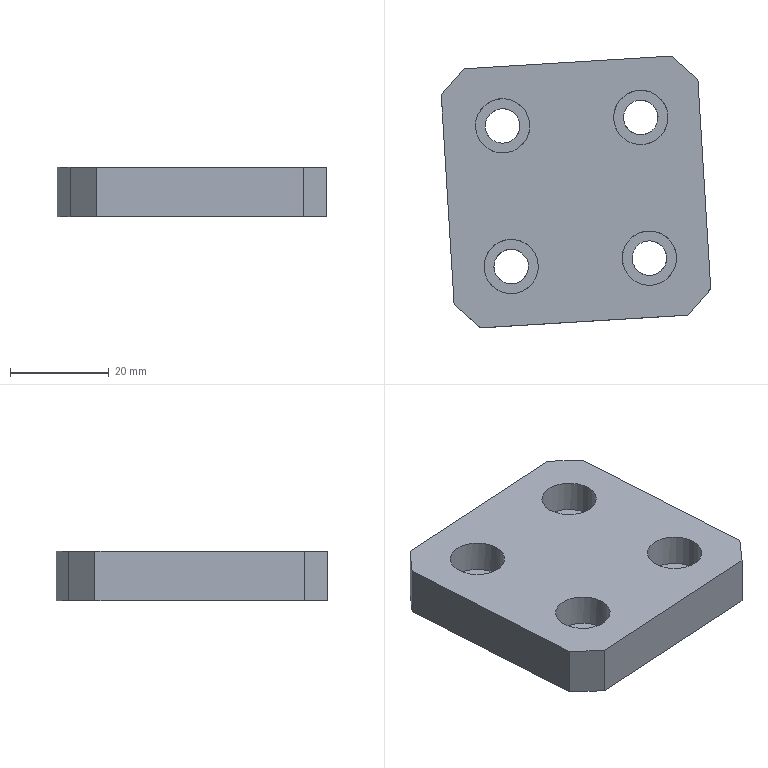Part | STEP file | 车灯-后视镜_id138_x_t | 1 solid | 22 faces | box 54.498 x 54.966 x 10 mm | volume 23790 mm3 | plane 14 | cylinder 8 | commonest cylinder face diameters 7 x4 11 x4
STEP:
#1=CARTESIAN_POINT('',(118.099,33.063,-255.5));
#2=VERTEX_POINT('',#1);
#3=CARTESIAN_POINT('',(120.693,-9.358,-255.5));
#4=VERTEX_POINT('',#3);
#5=CARTESIAN_POINT('',(119.355,12.524,-255.5));
#6=DIRECTION('',(0.06105,-0.9981,0.));
#7=VECTOR('',#6,1.);
#8=LINE('',#5,#7);
#9=EDGE_CURVE('',#2,#4,#8,.T.);
#10=ORIENTED_EDGE('',*,*,#9,.F.);
#11=CARTESIAN_POINT('',(112.803,37.748,-255.5));
#12=VERTEX_POINT('',#11);
#13=CARTESIAN_POINT('',(107.277,42.637,-255.5));
#14=DIRECTION('',(-0.749,0.6626,0.));
#15=VECTOR('',#14,1.);
#16=LINE('',#13,#15);
#17=EDGE_CURVE('',#2,#12,#16,.T.);
#18=ORIENTED_EDGE('',*,*,#17,.T.);
#19=CARTESIAN_POINT('',(70.881,35.184,-255.5));
#20=VERTEX_POINT('',#19);
#21=CARTESIAN_POINT('',(76.858,35.55,-255.5));
#22=DIRECTION('',(0.9981,0.06105,0.));
#23=VECTOR('',#22,1.);
#24=LINE('',#21,#23);
#25=EDGE_CURVE('',#20,#12,#24,.T.);
#26=ORIENTED_EDGE('',*,*,#25,.F.);
#27=CARTESIAN_POINT('',(66.196,29.888,-255.5));
#28=VERTEX_POINT('',#27);
#29=CARTESIAN_POINT('',(61.703,24.81,-255.5));
#30=DIRECTION('',(-0.6626,-0.749,0.));
#31=VECTOR('',#30,1.);
#32=LINE('',#29,#31);
#33=EDGE_CURVE('',#20,#28,#32,.T.);
#34=ORIENTED_EDGE('',*,*,#33,.T.);
#35=CARTESIAN_POINT('',(68.79,-12.533,-255.5));
#36=VERTEX_POINT('',#35);
#37=CARTESIAN_POINT('',(67.452,9.349,-255.5));
#38=DIRECTION('',(-0.06105,0.9981,0.));
#39=VECTOR('',#38,1.);
#40=LINE('',#37,#39);
#41=EDGE_CURVE('',#36,#28,#40,.T.);
#42=ORIENTED_EDGE('',*,*,#41,.F.);
#43=CARTESIAN_POINT('',(74.086,-17.218,-255.5));
#44=VERTEX_POINT('',#43);
#45=CARTESIAN_POINT('',(63.,-7.409,-255.5));
#46=DIRECTION('',(0.749,-0.6626,0.));
#47=VECTOR('',#46,1.);
#48=LINE('',#45,#47);
#49=EDGE_CURVE('',#36,#44,#48,.T.);
#50=ORIENTED_EDGE('',*,*,#49,.T.);
#51=CARTESIAN_POINT('',(116.008,-14.654,-255.5));
#52=VERTEX_POINT('',#51);
#53=CARTESIAN_POINT('',(80.063,-16.853,-255.5));
#54=DIRECTION('',(-0.9981,-0.06105,0.));
#55=VECTOR('',#54,1.);
#56=LINE('',#53,#55);
#57=EDGE_CURVE('',#52,#44,#56,.T.);
#58=ORIENTED_EDGE('',*,*,#57,.F.);
#59=CARTESIAN_POINT('',(111.749,-19.467,-255.5));
#60=DIRECTION('',(0.6626,0.749,0.));
#61=VECTOR('',#60,1.);
#62=LINE('',#59,#61);
#63=EDGE_CURVE('',#52,#4,#62,.T.);
#64=ORIENTED_EDGE('',*,*,#63,.T.);
#65=EDGE_LOOP('',(#10,#18,#26,#34,#42,#50,#58,#64));
#66=FACE_BOUND('',#65,.T.);
#67=CARTESIAN_POINT('',(85.841,-4.813,-255.5));
#68=VERTEX_POINT('',#67);
#69=CARTESIAN_POINT('',(80.341,-4.813,-255.5));
#70=DIRECTION('',(0.,0.,1.));
#71=DIRECTION('',(1.,0.,0.));
#72=AXIS2_PLACEMENT_3D('',#69,#70,#71);
#73=CIRCLE('',#72,5.5);
#74=EDGE_CURVE('',#68,#68,#73,.T.);
#75=ORIENTED_EDGE('',*,*,#74,.F.);
#76=EDGE_LOOP('',(#75));
#77=FACE_BOUND('',#76,.T.);
#78=CARTESIAN_POINT('',(113.788,-3.104,-255.5));
#79=VERTEX_POINT('',#78);
#80=CARTESIAN_POINT('',(108.288,-3.104,-255.5));
#81=DIRECTION('',(0.,0.,-1.));
#82=DIRECTION('',(1.,0.,0.));
#83=AXIS2_PLACEMENT_3D('',#80,#81,#82);
#84=CIRCLE('',#83,5.5);
#85=EDGE_CURVE('',#79,#79,#84,.T.);
#86=ORIENTED_EDGE('',*,*,#85,.T.);
#87=EDGE_LOOP('',(#86));
#88=FACE_BOUND('',#87,.T.);
#89=CARTESIAN_POINT('',(84.101,23.634,-255.5));
#90=VERTEX_POINT('',#89);
#91=CARTESIAN_POINT('',(78.601,23.634,-255.5));
#92=DIRECTION('',(0.,0.,-1.));
#93=DIRECTION('',(1.,0.,0.));
#94=AXIS2_PLACEMENT_3D('',#91,#92,#93);
#95=CIRCLE('',#94,5.5);
#96=EDGE_CURVE('',#90,#90,#95,.T.);
#97=ORIENTED_EDGE('',*,*,#96,.T.);
#98=EDGE_LOOP('',(#97));
#99=FACE_BOUND('',#98,.T.);
#100=CARTESIAN_POINT('',(112.049,25.343,-255.5));
#101=VERTEX_POINT('',#100);
#102=CARTESIAN_POINT('',(106.549,25.343,-255.5));
#103=DIRECTION('',(0.,0.,1.));
#104=DIRECTION('',(1.,0.,0.));
#105=AXIS2_PLACEMENT_3D('',#102,#103,#104);
#106=CIRCLE('',#105,5.5);
#107=EDGE_CURVE('',#101,#101,#106,.T.);
#108=ORIENTED_EDGE('',*,*,#107,.F.);
#109=EDGE_LOOP('',(#108));
#110=FACE_BOUND('',#109,.T.);
#111=CARTESIAN_POINT('',(78.42,10.02,-255.5));
#112=DIRECTION('',(0.,0.,1.));
#113=DIRECTION('',(0.9981,0.06105,0.));
#114=AXIS2_PLACEMENT_3D('',#111,#112,#113);
#115=PLANE('',#114);
#116=ADVANCED_FACE('',(#66,#77,#88,#99,#110),#115,.T.);
#117=CARTESIAN_POINT('',(74.086,-17.218,-265.5));
#118=VERTEX_POINT('',#117);
#119=CARTESIAN_POINT('',(116.008,-14.654,-265.5));
#120=VERTEX_POINT('',#119);
#121=CARTESIAN_POINT('',(80.063,-16.853,-265.5));
#122=DIRECTION('',(0.9981,0.06105,0.));
#123=VECTOR('',#122,1.);
#124=LINE('',#121,#123);
#125=EDGE_CURVE('',#118,#120,#124,.T.);
#126=ORIENTED_EDGE('',*,*,#125,.T.);
#127=CARTESIAN_POINT('',(116.008,-14.654,-267.5));
#128=DIRECTION('',(0.,0.,1.));
#129=VECTOR('',#128,1.);
#130=LINE('',#127,#129);
#131=EDGE_CURVE('',#120,#52,#130,.T.);
#132=ORIENTED_EDGE('',*,*,#131,.T.);
#133=ORIENTED_EDGE('',*,*,#57,.T.);
#134=CARTESIAN_POINT('',(74.086,-17.218,-267.5));
#135=DIRECTION('',(0.,0.,-1.));
#136=VECTOR('',#135,1.);
#137=LINE('',#134,#136);
#138=EDGE_CURVE('',#44,#118,#137,.T.);
#139=ORIENTED_EDGE('',*,*,#138,.T.);
#140=EDGE_LOOP('',(#126,#132,#133,#139));
#141=FACE_OUTER_BOUND('',#140,.T.);
#142=CARTESIAN_POINT('',(80.063,-16.853,-267.5));
#143=DIRECTION('',(0.06105,-0.9981,0.));
#144=DIRECTION('',(0.,0.,-1.));
#145=AXIS2_PLACEMENT_3D('',#142,#143,#144);
#146=PLANE('',#145);
#147=ADVANCED_FACE('',(#141),#146,.T.);
#148=ORIENTED_EDGE('',*,*,#25,.T.);
#149=CARTESIAN_POINT('',(112.803,37.748,-265.5));
#150=VERTEX_POINT('',#149);
#151=CARTESIAN_POINT('',(112.803,37.748,-267.5));
#152=DIRECTION('',(0.,0.,-1.));
#153=VECTOR('',#152,1.);
#154=LINE('',#151,#153);
#155=EDGE_CURVE('',#12,#150,#154,.T.);
#156=ORIENTED_EDGE('',*,*,#155,.T.);
#157=CARTESIAN_POINT('',(70.881,35.184,-265.5));
#158=VERTEX_POINT('',#157);
#159=CARTESIAN_POINT('',(76.858,35.55,-265.5));
#160=DIRECTION('',(-0.9981,-0.06105,0.));
#161=VECTOR('',#160,1.);
#162=LINE('',#159,#161);
#163=EDGE_CURVE('',#150,#158,#162,.T.);
#164=ORIENTED_EDGE('',*,*,#163,.T.);
#165=CARTESIAN_POINT('',(70.881,35.184,-267.5));
#166=DIRECTION('',(0.,0.,1.));
#167=VECTOR('',#166,1.);
#168=LINE('',#165,#167);
#169=EDGE_CURVE('',#158,#20,#168,.T.);
#170=ORIENTED_EDGE('',*,*,#169,.T.);
#171=EDGE_LOOP('',(#148,#156,#164,#170));
#172=FACE_OUTER_BOUND('',#171,.T.);
#173=CARTESIAN_POINT('',(76.858,35.55,-267.5));
#174=DIRECTION('',(-0.06105,0.9981,0.));
#175=DIRECTION('',(0.,0.,1.));
#176=AXIS2_PLACEMENT_3D('',#173,#174,#175);
#177=PLANE('',#176);
#178=ADVANCED_FACE('',(#172),#177,.T.);
#179=ORIENTED_EDGE('',*,*,#163,.F.);
#180=CARTESIAN_POINT('',(118.099,33.063,-265.5));
#181=VERTEX_POINT('',#180);
#182=CARTESIAN_POINT('',(107.277,42.637,-265.5));
#183=DIRECTION('',(0.749,-0.6626,0.));
#184=VECTOR('',#183,1.);
#185=LINE('',#182,#184);
#186=EDGE_CURVE('',#150,#181,#185,.T.);
#187=ORIENTED_EDGE('',*,*,#186,.T.);
#188=CARTESIAN_POINT('',(120.693,-9.358,-265.5));
#189=VERTEX_POINT('',#188);
#190=CARTESIAN_POINT('',(119.355,12.524,-265.5));
#191=DIRECTION('',(-0.06105,0.9981,0.));
#192=VECTOR('',#191,1.);
#193=LINE('',#190,#192);
#194=EDGE_CURVE('',#189,#181,#193,.T.);
#195=ORIENTED_EDGE('',*,*,#194,.F.);
#196=CARTESIAN_POINT('',(111.749,-19.467,-265.5));
#197=DIRECTION('',(-0.6626,-0.749,0.));
#198=VECTOR('',#197,1.);
#199=LINE('',#196,#198);
#200=EDGE_CURVE('',#189,#120,#199,.T.);
#201=ORIENTED_EDGE('',*,*,#200,.T.);
#202=ORIENTED_EDGE('',*,*,#125,.F.);
#203=CARTESIAN_POINT('',(68.79,-12.533,-265.5));
#204=VERTEX_POINT('',#203);
#205=CARTESIAN_POINT('',(63.,-7.409,-265.5));
#206=DIRECTION('',(-0.749,0.6626,0.));
#207=VECTOR('',#206,1.);
#208=LINE('',#205,#207);
#209=EDGE_CURVE('',#118,#204,#208,.T.);
#210=ORIENTED_EDGE('',*,*,#209,.T.);
#211=CARTESIAN_POINT('',(66.196,29.888,-265.5));
#212=VERTEX_POINT('',#211);
#213=CARTESIAN_POINT('',(67.452,9.349,-265.5));
#214=DIRECTION('',(0.06105,-0.9981,0.));
#215=VECTOR('',#214,1.);
#216=LINE('',#213,#215);
#217=EDGE_CURVE('',#212,#204,#216,.T.);
#218=ORIENTED_EDGE('',*,*,#217,.F.);
#219=CARTESIAN_POINT('',(61.703,24.81,-265.5));
#220=DIRECTION('',(0.6626,0.749,0.));
#221=VECTOR('',#220,1.);
#222=LINE('',#219,#221);
#223=EDGE_CURVE('',#212,#158,#222,.T.);
#224=ORIENTED_EDGE('',*,*,#223,.T.);
#225=EDGE_LOOP('',(#179,#187,#195,#201,#202,#210,#218,#224));
#226=FACE_BOUND('',#225,.T.);
#227=CARTESIAN_POINT('',(76.841,-4.813,-265.5));
#228=VERTEX_POINT('',#227);
#229=CARTESIAN_POINT('',(80.341,-4.813,-265.5));
#230=DIRECTION('',(0.,0.,-1.));
#231=DIRECTION('',(-1.,0.,0.));
#232=AXIS2_PLACEMENT_3D('',#229,#230,#231);
#233=CIRCLE('',#232,3.5);
#234=EDGE_CURVE('',#228,#228,#233,.T.);
#235=ORIENTED_EDGE('',*,*,#234,.F.);
#236=EDGE_LOOP('',(#235));
#237=FACE_BOUND('',#236,.T.);
#238=CARTESIAN_POINT('',(104.788,-3.104,-265.5));
#239=VERTEX_POINT('',#238);
#240=CARTESIAN_POINT('',(108.288,-3.104,-265.5));
#241=DIRECTION('',(0.,0.,1.));
#242=DIRECTION('',(-1.,0.,0.));
#243=AXIS2_PLACEMENT_3D('',#240,#241,#242);
#244=CIRCLE('',#243,3.5);
#245=EDGE_CURVE('',#239,#239,#244,.T.);
#246=ORIENTED_EDGE('',*,*,#245,.T.);
#247=EDGE_LOOP('',(#246));
#248=FACE_BOUND('',#247,.T.);
#249=CARTESIAN_POINT('',(75.101,23.634,-265.5));
#250=VERTEX_POINT('',#249);
#251=CARTESIAN_POINT('',(78.601,23.634,-265.5));
#252=DIRECTION('',(0.,0.,1.));
#253=DIRECTION('',(-1.,0.,0.));
#254=AXIS2_PLACEMENT_3D('',#251,#252,#253);
#255=CIRCLE('',#254,3.5);
#256=EDGE_CURVE('',#250,#250,#255,.T.);
#257=ORIENTED_EDGE('',*,*,#256,.T.);
#258=EDGE_LOOP('',(#257));
#259=FACE_BOUND('',#258,.T.);
#260=CARTESIAN_POINT('',(103.049,25.343,-265.5));
#261=VERTEX_POINT('',#260);
#262=CARTESIAN_POINT('',(106.549,25.343,-265.5));
#263=DIRECTION('',(0.,0.,-1.));
#264=DIRECTION('',(-1.,0.,0.));
#265=AXIS2_PLACEMENT_3D('',#262,#263,#264);
#266=CIRCLE('',#265,3.5);
#267=EDGE_CURVE('',#261,#261,#266,.T.);
#268=ORIENTED_EDGE('',*,*,#267,.F.);
#269=EDGE_LOOP('',(#268));
#270=FACE_BOUND('',#269,.T.);
#271=CARTESIAN_POINT('',(78.42,10.02,-265.5));
#272=DIRECTION('',(0.,0.,-1.));
#273=DIRECTION('',(-0.9981,-0.06105,0.));
#274=AXIS2_PLACEMENT_3D('',#271,#272,#273);
#275=PLANE('',#274);
#276=ADVANCED_FACE('',(#226,#237,#248,#259,#270),#275,.T.);
#277=ORIENTED_EDGE('',*,*,#194,.T.);
#278=CARTESIAN_POINT('',(118.099,33.063,-267.5));
#279=DIRECTION('',(0.,0.,1.));
#280=VECTOR('',#279,1.);
#281=LINE('',#278,#280);
#282=EDGE_CURVE('',#181,#2,#281,.T.);
#283=ORIENTED_EDGE('',*,*,#282,.T.);
#284=ORIENTED_EDGE('',*,*,#9,.T.);
#285=CARTESIAN_POINT('',(120.693,-9.358,-267.5));
#286=DIRECTION('',(0.,0.,-1.));
#287=VECTOR('',#286,1.);
#288=LINE('',#285,#287);
#289=EDGE_CURVE('',#4,#189,#288,.T.);
#290=ORIENTED_EDGE('',*,*,#289,.T.);
#291=EDGE_LOOP('',(#277,#283,#284,#290));
#292=FACE_OUTER_BOUND('',#291,.T.);
#293=CARTESIAN_POINT('',(119.355,12.524,-267.5));
#294=DIRECTION('',(0.9981,0.06105,0.));
#295=DIRECTION('',(0.,0.,-1.));
#296=AXIS2_PLACEMENT_3D('',#293,#294,#295);
#297=PLANE('',#296);
#298=ADVANCED_FACE('',(#292),#297,.T.);
#299=CARTESIAN_POINT('',(103.055,25.129,-262.));
#300=VERTEX_POINT('',#299);
#301=CARTESIAN_POINT('',(106.549,25.343,-262.));
#302=DIRECTION('',(0.,0.,-1.));
#303=DIRECTION('',(-0.9981,-0.06105,0.));
#304=AXIS2_PLACEMENT_3D('',#301,#302,#303);
#305=CIRCLE('',#304,3.5);
#306=EDGE_CURVE('',#300,#300,#305,.T.);
#307=ORIENTED_EDGE('',*,*,#306,.F.);
#308=EDGE_LOOP('',(#307));
#309=FACE_BOUND('',#308,.T.);
#310=ORIENTED_EDGE('',*,*,#267,.T.);
#311=EDGE_LOOP('',(#310));
#312=FACE_BOUND('',#311,.T.);
#313=CARTESIAN_POINT('',(106.549,25.343,-265.5));
#314=DIRECTION('',(0.,0.,1.));
#315=DIRECTION('',(-0.9981,-0.06105,0.));
#316=AXIS2_PLACEMENT_3D('',#313,#314,#315);
#317=CYLINDRICAL_SURFACE('',#316,3.5);
#318=ADVANCED_FACE('',(#309,#312),#317,.F.);
#319=ORIENTED_EDGE('',*,*,#306,.T.);
#320=EDGE_LOOP('',(#319));
#321=FACE_BOUND('',#320,.T.);
#322=CARTESIAN_POINT('',(101.059,25.007,-262.));
#323=VERTEX_POINT('',#322);
#324=CARTESIAN_POINT('',(106.549,25.343,-262.));
#325=DIRECTION('',(0.,0.,-1.));
#326=DIRECTION('',(-0.9981,-0.06105,0.));
#327=AXIS2_PLACEMENT_3D('',#324,#325,#326);
#328=CIRCLE('',#327,5.5);
#329=EDGE_CURVE('',#323,#323,#328,.T.);
#330=ORIENTED_EDGE('',*,*,#329,.F.);
#331=EDGE_LOOP('',(#330));
#332=FACE_BOUND('',#331,.T.);
#333=CARTESIAN_POINT('',(106.549,25.343,-262.));
#334=DIRECTION('',(0.,0.,-1.));
#335=DIRECTION('',(0.9981,0.06105,0.));
#336=AXIS2_PLACEMENT_3D('',#333,#334,#335);
#337=PLANE('',#336);
#338=ADVANCED_FACE('',(#321,#332),#337,.F.);
#339=ORIENTED_EDGE('',*,*,#329,.T.);
#340=EDGE_LOOP('',(#339));
#341=FACE_BOUND('',#340,.T.);
#342=ORIENTED_EDGE('',*,*,#107,.T.);
#343=EDGE_LOOP('',(#342));
#344=FACE_BOUND('',#343,.T.);
#345=CARTESIAN_POINT('',(106.549,25.343,-255.5));
#346=DIRECTION('',(0.,0.,-1.));
#347=DIRECTION('',(0.9981,0.06105,0.));
#348=AXIS2_PLACEMENT_3D('',#345,#346,#347);
#349=CYLINDRICAL_SURFACE('',#348,5.5);
#350=ADVANCED_FACE('',(#341,#344),#349,.F.);
#351=CARTESIAN_POINT('',(75.107,23.42,-262.));
#352=VERTEX_POINT('',#351);
#353=CARTESIAN_POINT('',(78.601,23.634,-262.));
#354=DIRECTION('',(0.,0.,1.));
#355=DIRECTION('',(-0.9981,-0.06105,0.));
#356=AXIS2_PLACEMENT_3D('',#353,#354,#355);
#357=CIRCLE('',#356,3.5);
#358=EDGE_CURVE('',#352,#352,#357,.T.);
#359=ORIENTED_EDGE('',*,*,#358,.T.);
#360=EDGE_LOOP('',(#359));
#361=FACE_BOUND('',#360,.T.);
#362=ORIENTED_EDGE('',*,*,#256,.F.);
#363=EDGE_LOOP('',(#362));
#364=FACE_BOUND('',#363,.T.);
#365=CARTESIAN_POINT('',(78.601,23.634,-265.5));
#366=DIRECTION('',(0.,0.,1.));
#367=DIRECTION('',(0.9981,0.06105,0.));
#368=AXIS2_PLACEMENT_3D('',#365,#366,#367);
#369=CYLINDRICAL_SURFACE('',#368,3.5);
#370=ADVANCED_FACE('',(#361,#364),#369,.F.);
#371=ORIENTED_EDGE('',*,*,#358,.F.);
#372=EDGE_LOOP('',(#371));
#373=FACE_BOUND('',#372,.T.);
#374=CARTESIAN_POINT('',(73.111,23.298,-262.));
#375=VERTEX_POINT('',#374);
#376=CARTESIAN_POINT('',(78.601,23.634,-262.));
#377=DIRECTION('',(0.,0.,1.));
#378=DIRECTION('',(-0.9981,-0.06105,0.));
#379=AXIS2_PLACEMENT_3D('',#376,#377,#378);
#380=CIRCLE('',#379,5.5);
#381=EDGE_CURVE('',#375,#375,#380,.T.);
#382=ORIENTED_EDGE('',*,*,#381,.T.);
#383=EDGE_LOOP('',(#382));
#384=FACE_BOUND('',#383,.T.);
#385=CARTESIAN_POINT('',(78.601,23.634,-262.));
#386=DIRECTION('',(0.,0.,-1.));
#387=DIRECTION('',(-0.9981,-0.06105,0.));
#388=AXIS2_PLACEMENT_3D('',#385,#386,#387);
#389=PLANE('',#388);
#390=ADVANCED_FACE('',(#373,#384),#389,.F.);
#391=ORIENTED_EDGE('',*,*,#381,.F.);
#392=EDGE_LOOP('',(#391));
#393=FACE_BOUND('',#392,.T.);
#394=ORIENTED_EDGE('',*,*,#96,.F.);
#395=EDGE_LOOP('',(#394));
#396=FACE_BOUND('',#395,.T.);
#397=CARTESIAN_POINT('',(78.601,23.634,-255.5));
#398=DIRECTION('',(0.,0.,-1.));
#399=DIRECTION('',(-0.9981,-0.06105,0.));
#400=AXIS2_PLACEMENT_3D('',#397,#398,#399);
#401=CYLINDRICAL_SURFACE('',#400,5.5);
#402=ADVANCED_FACE('',(#393,#396),#401,.F.);
#403=CARTESIAN_POINT('',(104.795,-3.317,-262.));
#404=VERTEX_POINT('',#403);
#405=CARTESIAN_POINT('',(108.288,-3.104,-262.));
#406=DIRECTION('',(0.,0.,1.));
#407=DIRECTION('',(-0.9981,-0.06105,0.));
#408=AXIS2_PLACEMENT_3D('',#405,#406,#407);
#409=CIRCLE('',#408,3.5);
#410=EDGE_CURVE('',#404,#404,#409,.T.);
#411=ORIENTED_EDGE('',*,*,#410,.T.);
#412=EDGE_LOOP('',(#411));
#413=FACE_BOUND('',#412,.T.);
#414=ORIENTED_EDGE('',*,*,#245,.F.);
#415=EDGE_LOOP('',(#414));
#416=FACE_BOUND('',#415,.T.);
#417=CARTESIAN_POINT('',(108.288,-3.104,-265.5));
#418=DIRECTION('',(0.,0.,1.));
#419=DIRECTION('',(-0.9981,-0.06105,0.));
#420=AXIS2_PLACEMENT_3D('',#417,#418,#419);
#421=CYLINDRICAL_SURFACE('',#420,3.5);
#422=ADVANCED_FACE('',(#413,#416),#421,.F.);
#423=ORIENTED_EDGE('',*,*,#410,.F.);
#424=EDGE_LOOP('',(#423));
#425=FACE_BOUND('',#424,.T.);
#426=CARTESIAN_POINT('',(102.799,-3.44,-262.));
#427=VERTEX_POINT('',#426);
#428=CARTESIAN_POINT('',(108.288,-3.104,-262.));
#429=DIRECTION('',(0.,0.,1.));
#430=DIRECTION('',(-0.9981,-0.06105,0.));
#431=AXIS2_PLACEMENT_3D('',#428,#429,#430);
#432=CIRCLE('',#431,5.5);
#433=EDGE_CURVE('',#427,#427,#432,.T.);
#434=ORIENTED_EDGE('',*,*,#433,.T.);
#435=EDGE_LOOP('',(#434));
#436=FACE_BOUND('',#435,.T.);
#437=CARTESIAN_POINT('',(108.288,-3.104,-262.));
#438=DIRECTION('',(0.,0.,-1.));
#439=DIRECTION('',(0.9981,0.06105,0.));
#440=AXIS2_PLACEMENT_3D('',#437,#438,#439);
#441=PLANE('',#440);
#442=ADVANCED_FACE('',(#425,#436),#441,.F.);
#443=ORIENTED_EDGE('',*,*,#433,.F.);
#444=EDGE_LOOP('',(#443));
#445=FACE_BOUND('',#444,.T.);
#446=ORIENTED_EDGE('',*,*,#85,.F.);
#447=EDGE_LOOP('',(#446));
#448=FACE_BOUND('',#447,.T.);
#449=CARTESIAN_POINT('',(108.288,-3.104,-255.5));
#450=DIRECTION('',(0.,0.,-1.));
#451=DIRECTION('',(0.9981,0.06105,0.));
#452=AXIS2_PLACEMENT_3D('',#449,#450,#451);
#453=CYLINDRICAL_SURFACE('',#452,5.5);
#454=ADVANCED_FACE('',(#445,#448),#453,.F.);
#455=CARTESIAN_POINT('',(76.847,-5.027,-262.));
#456=VERTEX_POINT('',#455);
#457=CARTESIAN_POINT('',(80.341,-4.813,-262.));
#458=DIRECTION('',(0.,0.,-1.));
#459=DIRECTION('',(-0.9981,-0.06105,0.));
#460=AXIS2_PLACEMENT_3D('',#457,#458,#459);
#461=CIRCLE('',#460,3.5);
#462=EDGE_CURVE('',#456,#456,#461,.T.);
#463=ORIENTED_EDGE('',*,*,#462,.F.);
#464=EDGE_LOOP('',(#463));
#465=FACE_BOUND('',#464,.T.);
#466=ORIENTED_EDGE('',*,*,#234,.T.);
#467=EDGE_LOOP('',(#466));
#468=FACE_BOUND('',#467,.T.);
#469=CARTESIAN_POINT('',(80.341,-4.813,-265.5));
#470=DIRECTION('',(0.,0.,1.));
#471=DIRECTION('',(0.9981,0.06105,0.));
#472=AXIS2_PLACEMENT_3D('',#469,#470,#471);
#473=CYLINDRICAL_SURFACE('',#472,3.5);
#474=ADVANCED_FACE('',(#465,#468),#473,.F.);
#475=ORIENTED_EDGE('',*,*,#462,.T.);
#476=EDGE_LOOP('',(#475));
#477=FACE_BOUND('',#476,.T.);
#478=CARTESIAN_POINT('',(74.851,-5.149,-262.));
#479=VERTEX_POINT('',#478);
#480=CARTESIAN_POINT('',(80.341,-4.813,-262.));
#481=DIRECTION('',(0.,0.,-1.));
#482=DIRECTION('',(-0.9981,-0.06105,0.));
#483=AXIS2_PLACEMENT_3D('',#480,#481,#482);
#484=CIRCLE('',#483,5.5);
#485=EDGE_CURVE('',#479,#479,#484,.T.);
#486=ORIENTED_EDGE('',*,*,#485,.F.);
#487=EDGE_LOOP('',(#486));
#488=FACE_BOUND('',#487,.T.);
#489=CARTESIAN_POINT('',(80.341,-4.813,-262.));
#490=DIRECTION('',(0.,0.,-1.));
#491=DIRECTION('',(-0.9981,-0.06105,0.));
#492=AXIS2_PLACEMENT_3D('',#489,#490,#491);
#493=PLANE('',#492);
#494=ADVANCED_FACE('',(#477,#488),#493,.F.);
#495=ORIENTED_EDGE('',*,*,#485,.T.);
#496=EDGE_LOOP('',(#495));
#497=FACE_BOUND('',#496,.T.);
#498=ORIENTED_EDGE('',*,*,#74,.T.);
#499=EDGE_LOOP('',(#498));
#500=FACE_BOUND('',#499,.T.);
#501=CARTESIAN_POINT('',(80.341,-4.813,-255.5));
#502=DIRECTION('',(0.,0.,-1.));
#503=DIRECTION('',(-0.9981,-0.06105,0.));
#504=AXIS2_PLACEMENT_3D('',#501,#502,#503);
#505=CYLINDRICAL_SURFACE('',#504,5.5);
#506=ADVANCED_FACE('',(#497,#500),#505,.F.);
#507=ORIENTED_EDGE('',*,*,#217,.T.);
#508=CARTESIAN_POINT('',(68.79,-12.533,-261.5));
#509=DIRECTION('',(0.,0.,1.));
#510=VECTOR('',#509,1.);
#511=LINE('',#508,#510);
#512=EDGE_CURVE('',#204,#36,#511,.T.);
#513=ORIENTED_EDGE('',*,*,#512,.T.);
#514=ORIENTED_EDGE('',*,*,#41,.T.);
#515=CARTESIAN_POINT('',(66.196,29.888,-261.5));
#516=DIRECTION('',(0.,0.,-1.));
#517=VECTOR('',#516,1.);
#518=LINE('',#515,#517);
#519=EDGE_CURVE('',#28,#212,#518,.T.);
#520=ORIENTED_EDGE('',*,*,#519,.T.);
#521=EDGE_LOOP('',(#507,#513,#514,#520));
#522=FACE_OUTER_BOUND('',#521,.T.);
#523=CARTESIAN_POINT('',(67.452,9.349,-261.5));
#524=DIRECTION('',(0.9981,0.06105,0.));
#525=DIRECTION('',(0.,0.,1.));
#526=AXIS2_PLACEMENT_3D('',#523,#524,#525);
#527=PLANE('',#526);
#528=ADVANCED_FACE('',(#522),#527,.F.);
#529=ORIENTED_EDGE('',*,*,#209,.F.);
#530=ORIENTED_EDGE('',*,*,#138,.F.);
#531=ORIENTED_EDGE('',*,*,#49,.F.);
#532=ORIENTED_EDGE('',*,*,#512,.F.);
#533=EDGE_LOOP('',(#529,#530,#531,#532));
#534=FACE_OUTER_BOUND('',#533,.T.);
#535=CARTESIAN_POINT('',(68.79,-12.533,-261.5));
#536=DIRECTION('',(-0.6626,-0.749,0.));
#537=DIRECTION('',(0.749,-0.6626,0.));
#538=AXIS2_PLACEMENT_3D('',#535,#536,#537);
#539=PLANE('',#538);
#540=ADVANCED_FACE('',(#534),#539,.T.);
#541=ORIENTED_EDGE('',*,*,#33,.F.);
#542=ORIENTED_EDGE('',*,*,#169,.F.);
#543=ORIENTED_EDGE('',*,*,#223,.F.);
#544=ORIENTED_EDGE('',*,*,#519,.F.);
#545=EDGE_LOOP('',(#541,#542,#543,#544));
#546=FACE_OUTER_BOUND('',#545,.T.);
#547=CARTESIAN_POINT('',(66.196,29.888,-261.5));
#548=DIRECTION('',(-0.749,0.6626,0.));
#549=DIRECTION('',(-0.6626,-0.749,0.));
#550=AXIS2_PLACEMENT_3D('',#547,#548,#549);
#551=PLANE('',#550);
#552=ADVANCED_FACE('',(#546),#551,.T.);
#553=ORIENTED_EDGE('',*,*,#17,.F.);
#554=ORIENTED_EDGE('',*,*,#282,.F.);
#555=ORIENTED_EDGE('',*,*,#186,.F.);
#556=ORIENTED_EDGE('',*,*,#155,.F.);
#557=EDGE_LOOP('',(#553,#554,#555,#556));
#558=FACE_OUTER_BOUND('',#557,.T.);
#559=CARTESIAN_POINT('',(112.803,37.748,-267.5));
#560=DIRECTION('',(-0.6626,-0.749,0.));
#561=DIRECTION('',(0.749,-0.6626,0.));
#562=AXIS2_PLACEMENT_3D('',#559,#560,#561);
#563=PLANE('',#562);
#564=ADVANCED_FACE('',(#558),#563,.F.);
#565=ORIENTED_EDGE('',*,*,#63,.F.);
#566=ORIENTED_EDGE('',*,*,#131,.F.);
#567=ORIENTED_EDGE('',*,*,#200,.F.);
#568=ORIENTED_EDGE('',*,*,#289,.F.);
#569=EDGE_LOOP('',(#565,#566,#567,#568));
#570=FACE_OUTER_BOUND('',#569,.T.);
#571=CARTESIAN_POINT('',(120.693,-9.358,-267.5));
#572=DIRECTION('',(-0.749,0.6626,0.));
#573=DIRECTION('',(-0.6626,-0.749,0.));
#574=AXIS2_PLACEMENT_3D('',#571,#572,#573);
#575=PLANE('',#574);
#576=ADVANCED_FACE('',(#570),#575,.F.);
#577=CLOSED_SHELL('',(#116,#147,#178,#276,#298,#318,#338,#350,#370,#390,#402,#422,#442,#454,#474,#494,#506,#528,#540,#552,#564,#576));
#578=MANIFOLD_SOLID_BREP('',#577);
#579=(LENGTH_UNIT()NAMED_UNIT(*)SI_UNIT(.MILLI.,.METRE.));
#580=UNCERTAINTY_MEASURE_WITH_UNIT(LENGTH_MEASURE(0.00002),#579,'','');
#581=(NAMED_UNIT(*)PLANE_ANGLE_UNIT()SI_UNIT($,.RADIAN.));
#582=PLANE_ANGLE_MEASURE_WITH_UNIT(PLANE_ANGLE_MEASURE(0.01745),#581);
#583=DIMENSIONAL_EXPONENTS(0.,0.,0.,0.,0.,0.,0.);
#584=(CONVERSION_BASED_UNIT('DEGREE',#582)NAMED_UNIT(#583)PLANE_ANGLE_UNIT());
#585=(NAMED_UNIT(*)SI_UNIT($,.STERADIAN.)SOLID_ANGLE_UNIT());
#586=(GEOMETRIC_REPRESENTATION_CONTEXT(3)GLOBAL_UNCERTAINTY_ASSIGNED_CONTEXT((#580))GLOBAL_UNIT_ASSIGNED_CONTEXT((#579,#584,#585))REPRESENTATION_CONTEXT('',''));
#587=ADVANCED_BREP_SHAPE_REPRESENTATION('',(#578),#586);